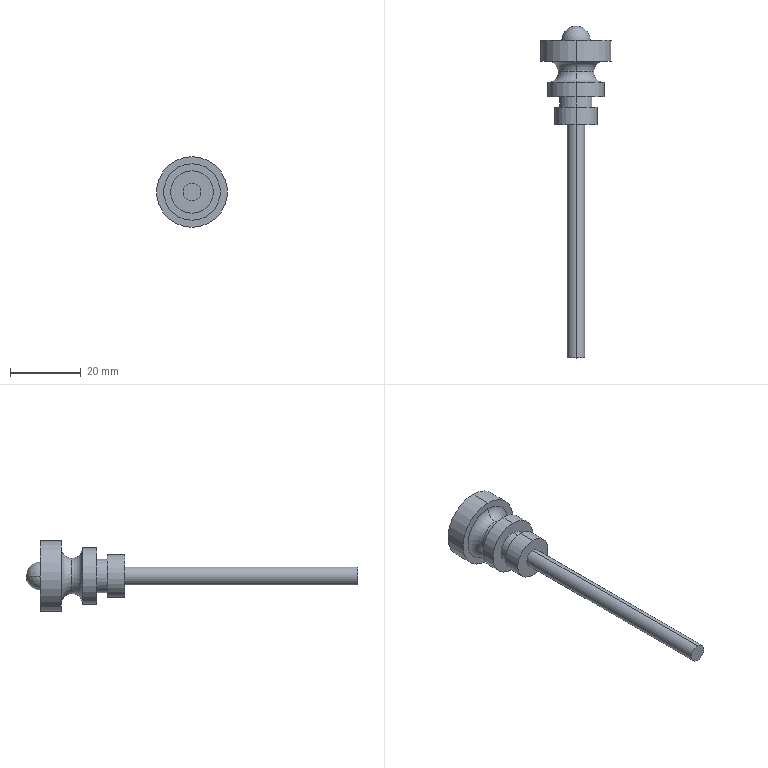Part | SolidWorks | features Revolution 2, RevCut 1 | 1 solid | 22 faces | box 20 x 94 x 20 mm | volume 5502 mm3 | cylinder 10 | plane 6 | torus 4 | sphere 2 | commonest cylinder face diameters 5 x2 9.4 x2 12 x2 16 x2 20 x2
STEP:
#1=CARTESIAN_POINT('',(0.,-6.,8.));
#2=VERTEX_POINT('',#1);
#3=CARTESIAN_POINT('',(0.,-9.,5.));
#4=VERTEX_POINT('',#3);
#5=CARTESIAN_POINT('',(0.,-9.,8.));
#6=DIRECTION('',(-1.,0.,0.));
#7=DIRECTION('',(0.,0.,1.));
#8=AXIS2_PLACEMENT_3D('',#5,#6,#7);
#9=CIRCLE('',#8,3.);
#10=EDGE_CURVE('',#2,#4,#9,.T.);
#11=ORIENTED_EDGE('',*,*,#10,.T.);
#12=CARTESIAN_POINT('',(0.,-9.,-5.));
#13=VERTEX_POINT('',#12);
#14=CARTESIAN_POINT('',(0.,-9.,0.));
#15=DIRECTION('',(0.,1.,0.));
#16=DIRECTION('',(0.,0.,1.));
#17=AXIS2_PLACEMENT_3D('',#14,#15,#16);
#18=CIRCLE('',#17,5.);
#19=EDGE_CURVE('',#4,#13,#18,.T.);
#20=ORIENTED_EDGE('',*,*,#19,.T.);
#21=CARTESIAN_POINT('',(0.,-6.,-8.));
#22=VERTEX_POINT('',#21);
#23=CARTESIAN_POINT('',(0.,-9.,-8.));
#24=DIRECTION('',(1.,0.,0.));
#25=DIRECTION('',(0.,0.,-1.));
#26=AXIS2_PLACEMENT_3D('',#23,#24,#25);
#27=CIRCLE('',#26,3.);
#28=EDGE_CURVE('',#22,#13,#27,.T.);
#29=ORIENTED_EDGE('',*,*,#28,.F.);
#30=CARTESIAN_POINT('',(0.,-6.,0.));
#31=DIRECTION('',(0.,1.,0.));
#32=DIRECTION('',(0.,0.,1.));
#33=AXIS2_PLACEMENT_3D('',#30,#31,#32);
#34=CIRCLE('',#33,8.);
#35=EDGE_CURVE('',#2,#22,#34,.T.);
#36=ORIENTED_EDGE('',*,*,#35,.F.);
#37=EDGE_LOOP('',(#11,#20,#29,#36));
#38=FACE_OUTER_BOUND('',#37,.T.);
#39=CARTESIAN_POINT('',(0.,-9.,0.));
#40=DIRECTION('',(0.,1.,0.));
#41=DIRECTION('',(0.,0.,1.));
#42=AXIS2_PLACEMENT_3D('',#39,#40,#41);
#43=TOROIDAL_SURFACE('',#42,8.,3.);
#44=ADVANCED_FACE('',(#38),#43,.F.);
#45=ORIENTED_EDGE('',*,*,#28,.T.);
#46=CARTESIAN_POINT('',(0.,-9.,0.));
#47=DIRECTION('',(0.,1.,0.));
#48=DIRECTION('',(0.,0.,1.));
#49=AXIS2_PLACEMENT_3D('',#46,#47,#48);
#50=CIRCLE('',#49,5.);
#51=EDGE_CURVE('',#13,#4,#50,.T.);
#52=ORIENTED_EDGE('',*,*,#51,.T.);
#53=ORIENTED_EDGE('',*,*,#10,.F.);
#54=CARTESIAN_POINT('',(0.,-6.,0.));
#55=DIRECTION('',(0.,1.,0.));
#56=DIRECTION('',(0.,0.,1.));
#57=AXIS2_PLACEMENT_3D('',#54,#55,#56);
#58=CIRCLE('',#57,8.);
#59=EDGE_CURVE('',#22,#2,#58,.T.);
#60=ORIENTED_EDGE('',*,*,#59,.F.);
#61=EDGE_LOOP('',(#45,#52,#53,#60));
#62=FACE_OUTER_BOUND('',#61,.T.);
#63=CARTESIAN_POINT('',(0.,-9.,0.));
#64=DIRECTION('',(0.,1.,0.));
#65=DIRECTION('',(0.,0.,1.));
#66=AXIS2_PLACEMENT_3D('',#63,#64,#65);
#67=TOROIDAL_SURFACE('',#66,8.,3.);
#68=ADVANCED_FACE('',(#62),#67,.F.);
#69=CARTESIAN_POINT('',(4.,0.,0.));
#70=VERTEX_POINT('',#69);
#71=CARTESIAN_POINT('',(-4.,0.,0.));
#72=VERTEX_POINT('',#71);
#73=CARTESIAN_POINT('',(0.,0.,0.));
#74=DIRECTION('',(0.,1.,0.));
#75=DIRECTION('',(-1.,0.,0.));
#76=AXIS2_PLACEMENT_3D('',#73,#74,#75);
#77=CIRCLE('',#76,4.);
#78=EDGE_CURVE('',#70,#72,#77,.T.);
#79=ORIENTED_EDGE('',*,*,#78,.T.);
#80=CARTESIAN_POINT('',(0.,4.,0.));
#81=VERTEX_POINT('',#80);
#82=CARTESIAN_POINT('',(0.,0.,0.));
#83=DIRECTION('',(0.,0.,-1.));
#84=DIRECTION('',(-1.,0.,0.));
#85=AXIS2_PLACEMENT_3D('',#82,#83,#84);
#86=CIRCLE('',#85,4.);
#87=EDGE_CURVE('',#72,#81,#86,.T.);
#88=ORIENTED_EDGE('',*,*,#87,.T.);
#89=CARTESIAN_POINT('',(0.,0.,0.));
#90=DIRECTION('',(0.,0.,1.));
#91=DIRECTION('',(1.,0.,0.));
#92=AXIS2_PLACEMENT_3D('',#89,#90,#91);
#93=CIRCLE('',#92,4.);
#94=EDGE_CURVE('',#70,#81,#93,.T.);
#95=ORIENTED_EDGE('',*,*,#94,.F.);
#96=EDGE_LOOP('',(#79,#88,#95));
#97=FACE_OUTER_BOUND('',#96,.T.);
#98=CARTESIAN_POINT('',(0.,0.,0.));
#99=DIRECTION('',(0.,0.,-1.));
#100=DIRECTION('',(1.,0.,0.));
#101=AXIS2_PLACEMENT_3D('',#98,#99,#100);
#102=SPHERICAL_SURFACE('',#101,4.);
#103=ADVANCED_FACE('',(#97),#102,.T.);
#104=CARTESIAN_POINT('',(0.,0.,-10.));
#105=VERTEX_POINT('',#104);
#106=CARTESIAN_POINT('',(0.,0.,10.));
#107=VERTEX_POINT('',#106);
#108=CARTESIAN_POINT('',(0.,0.,0.));
#109=DIRECTION('',(0.,-1.,0.));
#110=DIRECTION('',(0.,0.,-1.));
#111=AXIS2_PLACEMENT_3D('',#108,#109,#110);
#112=CIRCLE('',#111,10.);
#113=EDGE_CURVE('',#105,#107,#112,.T.);
#114=ORIENTED_EDGE('',*,*,#113,.T.);
#115=CARTESIAN_POINT('',(0.,-6.,10.));
#116=VERTEX_POINT('',#115);
#117=CARTESIAN_POINT('',(0.,0.,10.));
#118=DIRECTION('',(0.,-1.,0.));
#119=VECTOR('',#118,1000.);
#120=LINE('',#117,#119);
#121=EDGE_CURVE('',#107,#116,#120,.T.);
#122=ORIENTED_EDGE('',*,*,#121,.T.);
#123=CARTESIAN_POINT('',(0.,-6.,-10.));
#124=VERTEX_POINT('',#123);
#125=CARTESIAN_POINT('',(0.,-6.,0.));
#126=DIRECTION('',(0.,-1.,0.));
#127=DIRECTION('',(0.,0.,-1.));
#128=AXIS2_PLACEMENT_3D('',#125,#126,#127);
#129=CIRCLE('',#128,10.);
#130=EDGE_CURVE('',#124,#116,#129,.T.);
#131=ORIENTED_EDGE('',*,*,#130,.F.);
#132=CARTESIAN_POINT('',(0.,0.,-10.));
#133=DIRECTION('',(0.,-1.,0.));
#134=VECTOR('',#133,1000.);
#135=LINE('',#132,#134);
#136=EDGE_CURVE('',#105,#124,#135,.T.);
#137=ORIENTED_EDGE('',*,*,#136,.F.);
#138=EDGE_LOOP('',(#114,#122,#131,#137));
#139=FACE_OUTER_BOUND('',#138,.T.);
#140=CARTESIAN_POINT('',(0.,0.,0.));
#141=DIRECTION('',(0.,-1.,0.));
#142=DIRECTION('',(0.,0.,-1.));
#143=AXIS2_PLACEMENT_3D('',#140,#141,#142);
#144=CYLINDRICAL_SURFACE('',#143,10.);
#145=ADVANCED_FACE('',(#139),#144,.T.);
#146=ORIENTED_EDGE('',*,*,#51,.F.);
#147=CARTESIAN_POINT('',(0.,-12.,-8.));
#148=VERTEX_POINT('',#147);
#149=CARTESIAN_POINT('',(0.,-9.,-8.));
#150=DIRECTION('',(1.,0.,0.));
#151=DIRECTION('',(0.,0.,-1.));
#152=AXIS2_PLACEMENT_3D('',#149,#150,#151);
#153=CIRCLE('',#152,3.);
#154=EDGE_CURVE('',#13,#148,#153,.T.);
#155=ORIENTED_EDGE('',*,*,#154,.T.);
#156=CARTESIAN_POINT('',(0.,-12.,8.));
#157=VERTEX_POINT('',#156);
#158=CARTESIAN_POINT('',(0.,-12.,0.));
#159=DIRECTION('',(0.,1.,0.));
#160=DIRECTION('',(0.,0.,1.));
#161=AXIS2_PLACEMENT_3D('',#158,#159,#160);
#162=CIRCLE('',#161,8.);
#163=EDGE_CURVE('',#148,#157,#162,.T.);
#164=ORIENTED_EDGE('',*,*,#163,.T.);
#165=CARTESIAN_POINT('',(0.,-9.,8.));
#166=DIRECTION('',(-1.,0.,0.));
#167=DIRECTION('',(0.,0.,1.));
#168=AXIS2_PLACEMENT_3D('',#165,#166,#167);
#169=CIRCLE('',#168,3.);
#170=EDGE_CURVE('',#4,#157,#169,.T.);
#171=ORIENTED_EDGE('',*,*,#170,.F.);
#172=EDGE_LOOP('',(#146,#155,#164,#171));
#173=FACE_OUTER_BOUND('',#172,.T.);
#174=CARTESIAN_POINT('',(0.,-9.,0.));
#175=DIRECTION('',(0.,1.,0.));
#176=DIRECTION('',(0.,0.,1.));
#177=AXIS2_PLACEMENT_3D('',#174,#175,#176);
#178=TOROIDAL_SURFACE('',#177,8.,3.);
#179=ADVANCED_FACE('',(#173),#178,.F.);
#180=CARTESIAN_POINT('',(0.,-24.,-2.5));
#181=VERTEX_POINT('',#180);
#182=CARTESIAN_POINT('',(0.,-24.,2.5));
#183=VERTEX_POINT('',#182);
#184=CARTESIAN_POINT('',(0.,-24.,0.));
#185=DIRECTION('',(0.,-1.,0.));
#186=DIRECTION('',(0.,0.,-1.));
#187=AXIS2_PLACEMENT_3D('',#184,#185,#186);
#188=CIRCLE('',#187,2.5);
#189=EDGE_CURVE('',#181,#183,#188,.T.);
#190=ORIENTED_EDGE('',*,*,#189,.T.);
#191=CARTESIAN_POINT('',(0.,-90.,2.5));
#192=VERTEX_POINT('',#191);
#193=CARTESIAN_POINT('',(0.,0.,2.5));
#194=DIRECTION('',(0.,-1.,0.));
#195=VECTOR('',#194,1000.);
#196=LINE('',#193,#195);
#197=EDGE_CURVE('',#183,#192,#196,.T.);
#198=ORIENTED_EDGE('',*,*,#197,.T.);
#199=CARTESIAN_POINT('',(0.,-90.,-2.5));
#200=VERTEX_POINT('',#199);
#201=CARTESIAN_POINT('',(0.,-90.,0.));
#202=DIRECTION('',(0.,-1.,0.));
#203=DIRECTION('',(0.,0.,-1.));
#204=AXIS2_PLACEMENT_3D('',#201,#202,#203);
#205=CIRCLE('',#204,2.5);
#206=EDGE_CURVE('',#200,#192,#205,.T.);
#207=ORIENTED_EDGE('',*,*,#206,.F.);
#208=CARTESIAN_POINT('',(0.,0.,-2.5));
#209=DIRECTION('',(0.,-1.,0.));
#210=VECTOR('',#209,1000.);
#211=LINE('',#208,#210);
#212=EDGE_CURVE('',#181,#200,#211,.T.);
#213=ORIENTED_EDGE('',*,*,#212,.F.);
#214=EDGE_LOOP('',(#190,#198,#207,#213));
#215=FACE_OUTER_BOUND('',#214,.T.);
#216=CARTESIAN_POINT('',(0.,0.,0.));
#217=DIRECTION('',(0.,-1.,0.));
#218=DIRECTION('',(0.,0.,-1.));
#219=AXIS2_PLACEMENT_3D('',#216,#217,#218);
#220=CYLINDRICAL_SURFACE('',#219,2.5);
#221=ADVANCED_FACE('',(#215),#220,.T.);
#222=CARTESIAN_POINT('',(0.,-19.,-6.));
#223=VERTEX_POINT('',#222);
#224=CARTESIAN_POINT('',(0.,-19.,6.));
#225=VERTEX_POINT('',#224);
#226=CARTESIAN_POINT('',(0.,-19.,0.));
#227=DIRECTION('',(0.,-1.,0.));
#228=DIRECTION('',(0.,0.,-1.));
#229=AXIS2_PLACEMENT_3D('',#226,#227,#228);
#230=CIRCLE('',#229,6.);
#231=EDGE_CURVE('',#223,#225,#230,.T.);
#232=ORIENTED_EDGE('',*,*,#231,.T.);
#233=CARTESIAN_POINT('',(0.,-24.,6.));
#234=VERTEX_POINT('',#233);
#235=CARTESIAN_POINT('',(0.,0.,6.));
#236=DIRECTION('',(0.,-1.,0.));
#237=VECTOR('',#236,1000.);
#238=LINE('',#235,#237);
#239=EDGE_CURVE('',#225,#234,#238,.T.);
#240=ORIENTED_EDGE('',*,*,#239,.T.);
#241=CARTESIAN_POINT('',(0.,-24.,-6.));
#242=VERTEX_POINT('',#241);
#243=CARTESIAN_POINT('',(0.,-24.,0.));
#244=DIRECTION('',(0.,-1.,0.));
#245=DIRECTION('',(0.,0.,-1.));
#246=AXIS2_PLACEMENT_3D('',#243,#244,#245);
#247=CIRCLE('',#246,6.);
#248=EDGE_CURVE('',#242,#234,#247,.T.);
#249=ORIENTED_EDGE('',*,*,#248,.F.);
#250=CARTESIAN_POINT('',(0.,0.,-6.));
#251=DIRECTION('',(0.,-1.,0.));
#252=VECTOR('',#251,1000.);
#253=LINE('',#250,#252);
#254=EDGE_CURVE('',#223,#242,#253,.T.);
#255=ORIENTED_EDGE('',*,*,#254,.F.);
#256=EDGE_LOOP('',(#232,#240,#249,#255));
#257=FACE_OUTER_BOUND('',#256,.T.);
#258=CARTESIAN_POINT('',(0.,0.,0.));
#259=DIRECTION('',(0.,-1.,0.));
#260=DIRECTION('',(0.,0.,-1.));
#261=AXIS2_PLACEMENT_3D('',#258,#259,#260);
#262=CYLINDRICAL_SURFACE('',#261,6.);
#263=ADVANCED_FACE('',(#257),#262,.T.);
#264=CARTESIAN_POINT('',(0.,-16.,-4.7));
#265=VERTEX_POINT('',#264);
#266=CARTESIAN_POINT('',(0.,-16.,4.7));
#267=VERTEX_POINT('',#266);
#268=CARTESIAN_POINT('',(0.,-16.,0.));
#269=DIRECTION('',(0.,-1.,0.));
#270=DIRECTION('',(0.,0.,-1.));
#271=AXIS2_PLACEMENT_3D('',#268,#269,#270);
#272=CIRCLE('',#271,4.7);
#273=EDGE_CURVE('',#265,#267,#272,.T.);
#274=ORIENTED_EDGE('',*,*,#273,.T.);
#275=CARTESIAN_POINT('',(0.,-19.,4.7));
#276=VERTEX_POINT('',#275);
#277=CARTESIAN_POINT('',(0.,0.,4.7));
#278=DIRECTION('',(0.,-1.,0.));
#279=VECTOR('',#278,1000.);
#280=LINE('',#277,#279);
#281=EDGE_CURVE('',#267,#276,#280,.T.);
#282=ORIENTED_EDGE('',*,*,#281,.T.);
#283=CARTESIAN_POINT('',(0.,-19.,-4.7));
#284=VERTEX_POINT('',#283);
#285=CARTESIAN_POINT('',(0.,-19.,0.));
#286=DIRECTION('',(0.,-1.,0.));
#287=DIRECTION('',(0.,0.,-1.));
#288=AXIS2_PLACEMENT_3D('',#285,#286,#287);
#289=CIRCLE('',#288,4.7);
#290=EDGE_CURVE('',#284,#276,#289,.T.);
#291=ORIENTED_EDGE('',*,*,#290,.F.);
#292=CARTESIAN_POINT('',(0.,0.,-4.7));
#293=DIRECTION('',(0.,-1.,0.));
#294=VECTOR('',#293,1000.);
#295=LINE('',#292,#294);
#296=EDGE_CURVE('',#265,#284,#295,.T.);
#297=ORIENTED_EDGE('',*,*,#296,.F.);
#298=EDGE_LOOP('',(#274,#282,#291,#297));
#299=FACE_OUTER_BOUND('',#298,.T.);
#300=CARTESIAN_POINT('',(0.,0.,0.));
#301=DIRECTION('',(0.,-1.,0.));
#302=DIRECTION('',(0.,0.,-1.));
#303=AXIS2_PLACEMENT_3D('',#300,#301,#302);
#304=CYLINDRICAL_SURFACE('',#303,4.7);
#305=ADVANCED_FACE('',(#299),#304,.T.);
#306=CARTESIAN_POINT('',(0.,-12.,0.));
#307=DIRECTION('',(0.,1.,0.));
#308=DIRECTION('',(0.,0.,1.));
#309=AXIS2_PLACEMENT_3D('',#306,#307,#308);
#310=CIRCLE('',#309,8.);
#311=EDGE_CURVE('',#157,#148,#310,.T.);
#312=ORIENTED_EDGE('',*,*,#311,.F.);
#313=CARTESIAN_POINT('',(0.,-16.,8.));
#314=VERTEX_POINT('',#313);
#315=CARTESIAN_POINT('',(0.,0.,8.));
#316=DIRECTION('',(0.,-1.,0.));
#317=VECTOR('',#316,1000.);
#318=LINE('',#315,#317);
#319=EDGE_CURVE('',#157,#314,#318,.T.);
#320=ORIENTED_EDGE('',*,*,#319,.T.);
#321=CARTESIAN_POINT('',(0.,-16.,-8.));
#322=VERTEX_POINT('',#321);
#323=CARTESIAN_POINT('',(0.,-16.,0.));
#324=DIRECTION('',(0.,-1.,0.));
#325=DIRECTION('',(0.,0.,-1.));
#326=AXIS2_PLACEMENT_3D('',#323,#324,#325);
#327=CIRCLE('',#326,8.);
#328=EDGE_CURVE('',#322,#314,#327,.T.);
#329=ORIENTED_EDGE('',*,*,#328,.F.);
#330=CARTESIAN_POINT('',(0.,0.,-8.));
#331=DIRECTION('',(0.,-1.,0.));
#332=VECTOR('',#331,1000.);
#333=LINE('',#330,#332);
#334=EDGE_CURVE('',#148,#322,#333,.T.);
#335=ORIENTED_EDGE('',*,*,#334,.F.);
#336=EDGE_LOOP('',(#312,#320,#329,#335));
#337=FACE_OUTER_BOUND('',#336,.T.);
#338=CARTESIAN_POINT('',(0.,0.,0.));
#339=DIRECTION('',(0.,-1.,0.));
#340=DIRECTION('',(0.,0.,-1.));
#341=AXIS2_PLACEMENT_3D('',#338,#339,#340);
#342=CYLINDRICAL_SURFACE('',#341,8.);
#343=ADVANCED_FACE('',(#337),#342,.T.);
#344=ORIENTED_EDGE('',*,*,#319,.F.);
#345=ORIENTED_EDGE('',*,*,#163,.F.);
#346=ORIENTED_EDGE('',*,*,#334,.T.);
#347=CARTESIAN_POINT('',(0.,-16.,0.));
#348=DIRECTION('',(0.,-1.,0.));
#349=DIRECTION('',(0.,0.,-1.));
#350=AXIS2_PLACEMENT_3D('',#347,#348,#349);
#351=CIRCLE('',#350,8.);
#352=EDGE_CURVE('',#314,#322,#351,.T.);
#353=ORIENTED_EDGE('',*,*,#352,.F.);
#354=EDGE_LOOP('',(#344,#345,#346,#353));
#355=FACE_OUTER_BOUND('',#354,.T.);
#356=CARTESIAN_POINT('',(0.,0.,0.));
#357=DIRECTION('',(0.,-1.,0.));
#358=DIRECTION('',(0.,0.,-1.));
#359=AXIS2_PLACEMENT_3D('',#356,#357,#358);
#360=CYLINDRICAL_SURFACE('',#359,8.);
#361=ADVANCED_FACE('',(#355),#360,.T.);
#362=ORIENTED_EDGE('',*,*,#328,.T.);
#363=ORIENTED_EDGE('',*,*,#352,.T.);
#364=EDGE_LOOP('',(#362,#363));
#365=FACE_OUTER_BOUND('',#364,.T.);
#366=ORIENTED_EDGE('',*,*,#273,.F.);
#367=CARTESIAN_POINT('',(0.,-16.,0.));
#368=DIRECTION('',(0.,-1.,0.));
#369=DIRECTION('',(0.,0.,-1.));
#370=AXIS2_PLACEMENT_3D('',#367,#368,#369);
#371=CIRCLE('',#370,4.7);
#372=EDGE_CURVE('',#267,#265,#371,.T.);
#373=ORIENTED_EDGE('',*,*,#372,.F.);
#374=EDGE_LOOP('',(#366,#373));
#375=FACE_BOUND('',#374,.T.);
#376=CARTESIAN_POINT('',(8.,-16.,0.));
#377=DIRECTION('',(0.,-1.,0.));
#378=DIRECTION('',(0.,0.,-1.));
#379=AXIS2_PLACEMENT_3D('',#376,#377,#378);
#380=PLANE('',#379);
#381=ADVANCED_FACE('',(#365,#375),#380,.T.);
#382=ORIENTED_EDGE('',*,*,#281,.F.);
#383=ORIENTED_EDGE('',*,*,#372,.T.);
#384=ORIENTED_EDGE('',*,*,#296,.T.);
#385=CARTESIAN_POINT('',(0.,-19.,0.));
#386=DIRECTION('',(0.,-1.,0.));
#387=DIRECTION('',(0.,0.,-1.));
#388=AXIS2_PLACEMENT_3D('',#385,#386,#387);
#389=CIRCLE('',#388,4.7);
#390=EDGE_CURVE('',#276,#284,#389,.T.);
#391=ORIENTED_EDGE('',*,*,#390,.F.);
#392=EDGE_LOOP('',(#382,#383,#384,#391));
#393=FACE_OUTER_BOUND('',#392,.T.);
#394=CARTESIAN_POINT('',(0.,0.,0.));
#395=DIRECTION('',(0.,-1.,0.));
#396=DIRECTION('',(0.,0.,-1.));
#397=AXIS2_PLACEMENT_3D('',#394,#395,#396);
#398=CYLINDRICAL_SURFACE('',#397,4.7);
#399=ADVANCED_FACE('',(#393),#398,.T.);
#400=ORIENTED_EDGE('',*,*,#290,.T.);
#401=ORIENTED_EDGE('',*,*,#390,.T.);
#402=EDGE_LOOP('',(#400,#401));
#403=FACE_BOUND('',#402,.T.);
#404=ORIENTED_EDGE('',*,*,#231,.F.);
#405=CARTESIAN_POINT('',(0.,-19.,0.));
#406=DIRECTION('',(0.,-1.,0.));
#407=DIRECTION('',(0.,0.,-1.));
#408=AXIS2_PLACEMENT_3D('',#405,#406,#407);
#409=CIRCLE('',#408,6.);
#410=EDGE_CURVE('',#225,#223,#409,.T.);
#411=ORIENTED_EDGE('',*,*,#410,.F.);
#412=EDGE_LOOP('',(#404,#411));
#413=FACE_OUTER_BOUND('',#412,.T.);
#414=CARTESIAN_POINT('',(4.7,-19.,0.));
#415=DIRECTION('',(0.,1.,0.));
#416=DIRECTION('',(0.,0.,1.));
#417=AXIS2_PLACEMENT_3D('',#414,#415,#416);
#418=PLANE('',#417);
#419=ADVANCED_FACE('',(#403,#413),#418,.T.);
#420=ORIENTED_EDGE('',*,*,#239,.F.);
#421=ORIENTED_EDGE('',*,*,#410,.T.);
#422=ORIENTED_EDGE('',*,*,#254,.T.);
#423=CARTESIAN_POINT('',(0.,-24.,0.));
#424=DIRECTION('',(0.,-1.,0.));
#425=DIRECTION('',(0.,0.,-1.));
#426=AXIS2_PLACEMENT_3D('',#423,#424,#425);
#427=CIRCLE('',#426,6.);
#428=EDGE_CURVE('',#234,#242,#427,.T.);
#429=ORIENTED_EDGE('',*,*,#428,.F.);
#430=EDGE_LOOP('',(#420,#421,#422,#429));
#431=FACE_OUTER_BOUND('',#430,.T.);
#432=CARTESIAN_POINT('',(0.,0.,0.));
#433=DIRECTION('',(0.,-1.,0.));
#434=DIRECTION('',(0.,0.,-1.));
#435=AXIS2_PLACEMENT_3D('',#432,#433,#434);
#436=CYLINDRICAL_SURFACE('',#435,6.);
#437=ADVANCED_FACE('',(#431),#436,.T.);
#438=ORIENTED_EDGE('',*,*,#248,.T.);
#439=ORIENTED_EDGE('',*,*,#428,.T.);
#440=EDGE_LOOP('',(#438,#439));
#441=FACE_OUTER_BOUND('',#440,.T.);
#442=ORIENTED_EDGE('',*,*,#189,.F.);
#443=CARTESIAN_POINT('',(0.,-24.,0.));
#444=DIRECTION('',(0.,-1.,0.));
#445=DIRECTION('',(0.,0.,-1.));
#446=AXIS2_PLACEMENT_3D('',#443,#444,#445);
#447=CIRCLE('',#446,2.5);
#448=EDGE_CURVE('',#183,#181,#447,.T.);
#449=ORIENTED_EDGE('',*,*,#448,.F.);
#450=EDGE_LOOP('',(#442,#449));
#451=FACE_BOUND('',#450,.T.);
#452=CARTESIAN_POINT('',(6.,-24.,0.));
#453=DIRECTION('',(0.,-1.,0.));
#454=DIRECTION('',(0.,0.,-1.));
#455=AXIS2_PLACEMENT_3D('',#452,#453,#454);
#456=PLANE('',#455);
#457=ADVANCED_FACE('',(#441,#451),#456,.T.);
#458=ORIENTED_EDGE('',*,*,#197,.F.);
#459=ORIENTED_EDGE('',*,*,#448,.T.);
#460=ORIENTED_EDGE('',*,*,#212,.T.);
#461=CARTESIAN_POINT('',(0.,-90.,0.));
#462=DIRECTION('',(0.,-1.,0.));
#463=DIRECTION('',(0.,0.,-1.));
#464=AXIS2_PLACEMENT_3D('',#461,#462,#463);
#465=CIRCLE('',#464,2.5);
#466=EDGE_CURVE('',#192,#200,#465,.T.);
#467=ORIENTED_EDGE('',*,*,#466,.F.);
#468=EDGE_LOOP('',(#458,#459,#460,#467));
#469=FACE_OUTER_BOUND('',#468,.T.);
#470=CARTESIAN_POINT('',(0.,0.,0.));
#471=DIRECTION('',(0.,-1.,0.));
#472=DIRECTION('',(0.,0.,-1.));
#473=AXIS2_PLACEMENT_3D('',#470,#471,#472);
#474=CYLINDRICAL_SURFACE('',#473,2.5);
#475=ADVANCED_FACE('',(#469),#474,.T.);
#476=ORIENTED_EDGE('',*,*,#206,.T.);
#477=ORIENTED_EDGE('',*,*,#466,.T.);
#478=EDGE_LOOP('',(#476,#477));
#479=FACE_OUTER_BOUND('',#478,.T.);
#480=CARTESIAN_POINT('',(2.5,-90.,0.));
#481=DIRECTION('',(0.,-1.,0.));
#482=DIRECTION('',(0.,0.,-1.));
#483=AXIS2_PLACEMENT_3D('',#480,#481,#482);
#484=PLANE('',#483);
#485=ADVANCED_FACE('',(#479),#484,.T.);
#486=ORIENTED_EDGE('',*,*,#19,.F.);
#487=ORIENTED_EDGE('',*,*,#170,.T.);
#488=ORIENTED_EDGE('',*,*,#311,.T.);
#489=ORIENTED_EDGE('',*,*,#154,.F.);
#490=EDGE_LOOP('',(#486,#487,#488,#489));
#491=FACE_OUTER_BOUND('',#490,.T.);
#492=CARTESIAN_POINT('',(0.,-9.,0.));
#493=DIRECTION('',(0.,1.,0.));
#494=DIRECTION('',(0.,0.,1.));
#495=AXIS2_PLACEMENT_3D('',#492,#493,#494);
#496=TOROIDAL_SURFACE('',#495,8.,3.);
#497=ADVANCED_FACE('',(#491),#496,.F.);
#498=ORIENTED_EDGE('',*,*,#78,.F.);
#499=CARTESIAN_POINT('',(0.,0.,0.));
#500=DIRECTION('',(0.,1.,0.));
#501=DIRECTION('',(-1.,0.,0.));
#502=AXIS2_PLACEMENT_3D('',#499,#500,#501);
#503=CIRCLE('',#502,4.);
#504=EDGE_CURVE('',#72,#70,#503,.T.);
#505=ORIENTED_EDGE('',*,*,#504,.F.);
#506=EDGE_LOOP('',(#498,#505));
#507=FACE_BOUND('',#506,.T.);
#508=ORIENTED_EDGE('',*,*,#113,.F.);
#509=CARTESIAN_POINT('',(0.,0.,0.));
#510=DIRECTION('',(0.,-1.,0.));
#511=DIRECTION('',(0.,0.,-1.));
#512=AXIS2_PLACEMENT_3D('',#509,#510,#511);
#513=CIRCLE('',#512,10.);
#514=EDGE_CURVE('',#107,#105,#513,.T.);
#515=ORIENTED_EDGE('',*,*,#514,.F.);
#516=EDGE_LOOP('',(#508,#515));
#517=FACE_OUTER_BOUND('',#516,.T.);
#518=CARTESIAN_POINT('',(0.,0.,0.));
#519=DIRECTION('',(0.,1.,0.));
#520=DIRECTION('',(0.,0.,1.));
#521=AXIS2_PLACEMENT_3D('',#518,#519,#520);
#522=PLANE('',#521);
#523=ADVANCED_FACE('',(#507,#517),#522,.T.);
#524=ORIENTED_EDGE('',*,*,#121,.F.);
#525=ORIENTED_EDGE('',*,*,#514,.T.);
#526=ORIENTED_EDGE('',*,*,#136,.T.);
#527=CARTESIAN_POINT('',(0.,-6.,0.));
#528=DIRECTION('',(0.,-1.,0.));
#529=DIRECTION('',(0.,0.,-1.));
#530=AXIS2_PLACEMENT_3D('',#527,#528,#529);
#531=CIRCLE('',#530,10.);
#532=EDGE_CURVE('',#116,#124,#531,.T.);
#533=ORIENTED_EDGE('',*,*,#532,.F.);
#534=EDGE_LOOP('',(#524,#525,#526,#533));
#535=FACE_OUTER_BOUND('',#534,.T.);
#536=CARTESIAN_POINT('',(0.,0.,0.));
#537=DIRECTION('',(0.,-1.,0.));
#538=DIRECTION('',(0.,0.,-1.));
#539=AXIS2_PLACEMENT_3D('',#536,#537,#538);
#540=CYLINDRICAL_SURFACE('',#539,10.);
#541=ADVANCED_FACE('',(#535),#540,.T.);
#542=ORIENTED_EDGE('',*,*,#130,.T.);
#543=ORIENTED_EDGE('',*,*,#532,.T.);
#544=EDGE_LOOP('',(#542,#543));
#545=FACE_OUTER_BOUND('',#544,.T.);
#546=ORIENTED_EDGE('',*,*,#35,.T.);
#547=ORIENTED_EDGE('',*,*,#59,.T.);
#548=EDGE_LOOP('',(#546,#547));
#549=FACE_BOUND('',#548,.T.);
#550=CARTESIAN_POINT('',(10.,-6.,0.));
#551=DIRECTION('',(0.,-1.,0.));
#552=DIRECTION('',(0.,0.,-1.));
#553=AXIS2_PLACEMENT_3D('',#550,#551,#552);
#554=PLANE('',#553);
#555=ADVANCED_FACE('',(#545,#549),#554,.T.);
#556=ORIENTED_EDGE('',*,*,#87,.F.);
#557=ORIENTED_EDGE('',*,*,#504,.T.);
#558=ORIENTED_EDGE('',*,*,#94,.T.);
#559=EDGE_LOOP('',(#556,#557,#558));
#560=FACE_OUTER_BOUND('',#559,.T.);
#561=CARTESIAN_POINT('',(0.,0.,0.));
#562=DIRECTION('',(0.,0.,-1.));
#563=DIRECTION('',(1.,0.,0.));
#564=AXIS2_PLACEMENT_3D('',#561,#562,#563);
#565=SPHERICAL_SURFACE('',#564,4.);
#566=ADVANCED_FACE('',(#560),#565,.T.);
#567=CLOSED_SHELL('',(#44,#68,#103,#145,#179,#221,#263,#305,#343,#361,#381,#399,#419,#437,#457,#475,#485,#497,#523,#541,#555,#566));
#568=MANIFOLD_SOLID_BREP('',#567);
#569=CARTESIAN_POINT('',(0.,0.,0.));
#570=DIRECTION('',(0.,0.,1.));
#571=DIRECTION('',(1.,0.,0.));
#572=AXIS2_PLACEMENT_3D('',#569,#570,#571);
#573=(LENGTH_UNIT()NAMED_UNIT(*)SI_UNIT(.MILLI.,.METRE.));
#574=UNCERTAINTY_MEASURE_WITH_UNIT(LENGTH_MEASURE(0.00001),#573,'','');
#575=(NAMED_UNIT(*)PLANE_ANGLE_UNIT()SI_UNIT($,.RADIAN.));
#576=(NAMED_UNIT(*)SI_UNIT($,.STERADIAN.)SOLID_ANGLE_UNIT());
#577=(GEOMETRIC_REPRESENTATION_CONTEXT(3)GLOBAL_UNCERTAINTY_ASSIGNED_CONTEXT((#574))GLOBAL_UNIT_ASSIGNED_CONTEXT((#573,#575,#576))REPRESENTATION_CONTEXT('',''));
#578=ADVANCED_BREP_SHAPE_REPRESENTATION('',(#568,#572),#577);